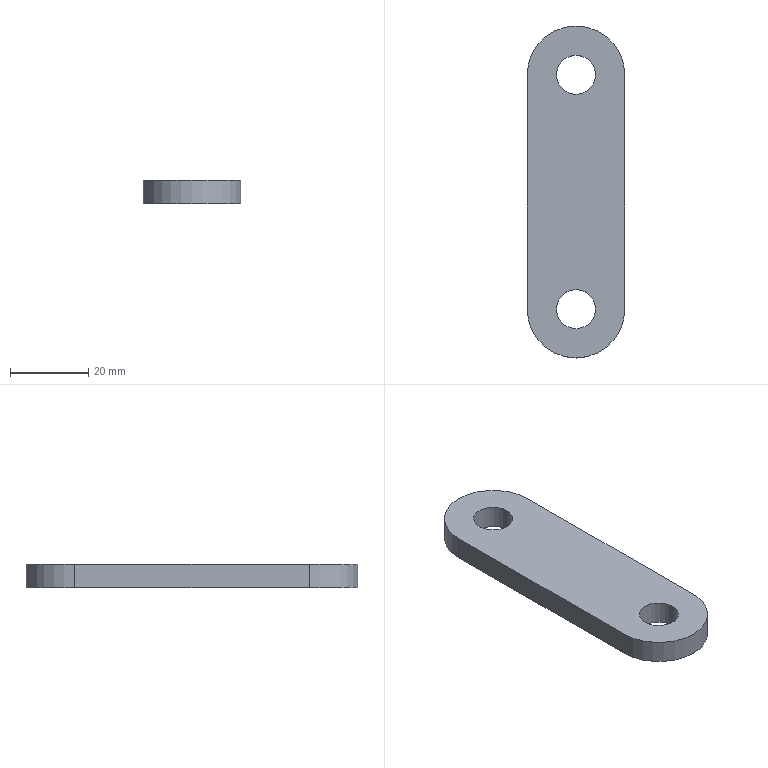Part | SolidWorks | features Extrusion 1 | 1 solid | 10 faces | box 25 x 85 x 6 mm | volume 11003 mm3 | cylinder 6 | plane 4 | commonest cylinder face diameters 10 x4 25 x2
STEP:
#1=CARTESIAN_POINT('',(-5.,60.,3.));
#2=VERTEX_POINT('',#1);
#3=CARTESIAN_POINT('',(5.,60.,3.));
#4=VERTEX_POINT('',#3);
#5=CARTESIAN_POINT('',(0.,60.,3.));
#6=DIRECTION('',(0.,0.,1.));
#7=DIRECTION('',(1.,0.,0.));
#8=AXIS2_PLACEMENT_3D('',#5,#6,#7);
#9=CIRCLE('',#8,5.);
#10=EDGE_CURVE('',#2,#4,#9,.T.);
#11=ORIENTED_EDGE('',*,*,#10,.T.);
#12=CARTESIAN_POINT('',(5.,60.,-3.));
#13=VERTEX_POINT('',#12);
#14=CARTESIAN_POINT('',(5.,60.,3.));
#15=DIRECTION('',(0.,0.,-1.));
#16=VECTOR('',#15,1000.);
#17=LINE('',#14,#16);
#18=EDGE_CURVE('',#4,#13,#17,.T.);
#19=ORIENTED_EDGE('',*,*,#18,.T.);
#20=CARTESIAN_POINT('',(-5.,60.,-3.));
#21=VERTEX_POINT('',#20);
#22=CARTESIAN_POINT('',(0.,60.,-3.));
#23=DIRECTION('',(0.,0.,1.));
#24=DIRECTION('',(1.,0.,0.));
#25=AXIS2_PLACEMENT_3D('',#22,#23,#24);
#26=CIRCLE('',#25,5.);
#27=EDGE_CURVE('',#21,#13,#26,.T.);
#28=ORIENTED_EDGE('',*,*,#27,.F.);
#29=CARTESIAN_POINT('',(-5.,60.,3.));
#30=DIRECTION('',(0.,0.,-1.));
#31=VECTOR('',#30,1000.);
#32=LINE('',#29,#31);
#33=EDGE_CURVE('',#2,#21,#32,.T.);
#34=ORIENTED_EDGE('',*,*,#33,.F.);
#35=EDGE_LOOP('',(#11,#19,#28,#34));
#36=FACE_OUTER_BOUND('',#35,.T.);
#37=CARTESIAN_POINT('',(0.,60.,3.));
#38=DIRECTION('',(0.,0.,-1.));
#39=DIRECTION('',(-1.,0.,0.));
#40=AXIS2_PLACEMENT_3D('',#37,#38,#39);
#41=CYLINDRICAL_SURFACE('',#40,5.);
#42=ADVANCED_FACE('',(#36),#41,.F.);
#43=CARTESIAN_POINT('',(-5.,0.,3.));
#44=VERTEX_POINT('',#43);
#45=CARTESIAN_POINT('',(5.,0.,3.));
#46=VERTEX_POINT('',#45);
#47=CARTESIAN_POINT('',(0.,0.,3.));
#48=DIRECTION('',(0.,0.,1.));
#49=DIRECTION('',(1.,0.,0.));
#50=AXIS2_PLACEMENT_3D('',#47,#48,#49);
#51=CIRCLE('',#50,5.);
#52=EDGE_CURVE('',#44,#46,#51,.T.);
#53=ORIENTED_EDGE('',*,*,#52,.T.);
#54=CARTESIAN_POINT('',(5.,0.,-3.));
#55=VERTEX_POINT('',#54);
#56=CARTESIAN_POINT('',(5.,0.,3.));
#57=DIRECTION('',(0.,0.,-1.));
#58=VECTOR('',#57,1000.);
#59=LINE('',#56,#58);
#60=EDGE_CURVE('',#46,#55,#59,.T.);
#61=ORIENTED_EDGE('',*,*,#60,.T.);
#62=CARTESIAN_POINT('',(-5.,0.,-3.));
#63=VERTEX_POINT('',#62);
#64=CARTESIAN_POINT('',(0.,0.,-3.));
#65=DIRECTION('',(0.,0.,1.));
#66=DIRECTION('',(1.,0.,0.));
#67=AXIS2_PLACEMENT_3D('',#64,#65,#66);
#68=CIRCLE('',#67,5.);
#69=EDGE_CURVE('',#63,#55,#68,.T.);
#70=ORIENTED_EDGE('',*,*,#69,.F.);
#71=CARTESIAN_POINT('',(-5.,0.,3.));
#72=DIRECTION('',(0.,0.,-1.));
#73=VECTOR('',#72,1000.);
#74=LINE('',#71,#73);
#75=EDGE_CURVE('',#44,#63,#74,.T.);
#76=ORIENTED_EDGE('',*,*,#75,.F.);
#77=EDGE_LOOP('',(#53,#61,#70,#76));
#78=FACE_OUTER_BOUND('',#77,.T.);
#79=CARTESIAN_POINT('',(0.,0.,3.));
#80=DIRECTION('',(0.,0.,-1.));
#81=DIRECTION('',(-1.,0.,0.));
#82=AXIS2_PLACEMENT_3D('',#79,#80,#81);
#83=CYLINDRICAL_SURFACE('',#82,5.);
#84=ADVANCED_FACE('',(#78),#83,.F.);
#85=ORIENTED_EDGE('',*,*,#52,.F.);
#86=CARTESIAN_POINT('',(0.,0.,3.));
#87=DIRECTION('',(0.,0.,1.));
#88=DIRECTION('',(1.,0.,0.));
#89=AXIS2_PLACEMENT_3D('',#86,#87,#88);
#90=CIRCLE('',#89,5.);
#91=EDGE_CURVE('',#46,#44,#90,.T.);
#92=ORIENTED_EDGE('',*,*,#91,.F.);
#93=EDGE_LOOP('',(#85,#92));
#94=FACE_BOUND('',#93,.T.);
#95=CARTESIAN_POINT('',(-12.5,0.,3.));
#96=VERTEX_POINT('',#95);
#97=CARTESIAN_POINT('',(12.5,0.,3.));
#98=VERTEX_POINT('',#97);
#99=CARTESIAN_POINT('',(0.,0.,3.));
#100=DIRECTION('',(0.,0.,1.));
#101=DIRECTION('',(1.,0.,0.));
#102=AXIS2_PLACEMENT_3D('',#99,#100,#101);
#103=CIRCLE('',#102,12.5);
#104=EDGE_CURVE('',#96,#98,#103,.T.);
#105=ORIENTED_EDGE('',*,*,#104,.T.);
#106=CARTESIAN_POINT('',(12.5,60.,3.));
#107=VERTEX_POINT('',#106);
#108=CARTESIAN_POINT('',(12.5,0.,3.));
#109=DIRECTION('',(0.,1.,0.));
#110=VECTOR('',#109,1000.);
#111=LINE('',#108,#110);
#112=EDGE_CURVE('',#98,#107,#111,.T.);
#113=ORIENTED_EDGE('',*,*,#112,.T.);
#114=CARTESIAN_POINT('',(-12.5,60.,3.));
#115=VERTEX_POINT('',#114);
#116=CARTESIAN_POINT('',(0.,60.,3.));
#117=DIRECTION('',(0.,0.,1.));
#118=DIRECTION('',(1.,0.,0.));
#119=AXIS2_PLACEMENT_3D('',#116,#117,#118);
#120=CIRCLE('',#119,12.5);
#121=EDGE_CURVE('',#107,#115,#120,.T.);
#122=ORIENTED_EDGE('',*,*,#121,.T.);
#123=CARTESIAN_POINT('',(-12.5,0.,3.));
#124=DIRECTION('',(0.,-1.,0.));
#125=VECTOR('',#124,1000.);
#126=LINE('',#123,#125);
#127=EDGE_CURVE('',#115,#96,#126,.T.);
#128=ORIENTED_EDGE('',*,*,#127,.T.);
#129=EDGE_LOOP('',(#105,#113,#122,#128));
#130=FACE_OUTER_BOUND('',#129,.T.);
#131=ORIENTED_EDGE('',*,*,#10,.F.);
#132=CARTESIAN_POINT('',(0.,60.,3.));
#133=DIRECTION('',(0.,0.,1.));
#134=DIRECTION('',(1.,0.,0.));
#135=AXIS2_PLACEMENT_3D('',#132,#133,#134);
#136=CIRCLE('',#135,5.);
#137=EDGE_CURVE('',#4,#2,#136,.T.);
#138=ORIENTED_EDGE('',*,*,#137,.F.);
#139=EDGE_LOOP('',(#131,#138));
#140=FACE_BOUND('',#139,.T.);
#141=CARTESIAN_POINT('',(0.,0.,3.));
#142=DIRECTION('',(0.,0.,1.));
#143=DIRECTION('',(1.,0.,0.));
#144=AXIS2_PLACEMENT_3D('',#141,#142,#143);
#145=PLANE('',#144);
#146=ADVANCED_FACE('',(#94,#130,#140),#145,.T.);
#147=CARTESIAN_POINT('',(-12.5,0.,-3.));
#148=VERTEX_POINT('',#147);
#149=CARTESIAN_POINT('',(12.5,0.,-3.));
#150=VERTEX_POINT('',#149);
#151=CARTESIAN_POINT('',(0.,0.,-3.));
#152=DIRECTION('',(0.,0.,1.));
#153=DIRECTION('',(1.,0.,0.));
#154=AXIS2_PLACEMENT_3D('',#151,#152,#153);
#155=CIRCLE('',#154,12.5);
#156=EDGE_CURVE('',#148,#150,#155,.T.);
#157=ORIENTED_EDGE('',*,*,#156,.F.);
#158=CARTESIAN_POINT('',(-12.5,60.,-3.));
#159=VERTEX_POINT('',#158);
#160=CARTESIAN_POINT('',(-12.5,0.,-3.));
#161=DIRECTION('',(0.,-1.,0.));
#162=VECTOR('',#161,1000.);
#163=LINE('',#160,#162);
#164=EDGE_CURVE('',#159,#148,#163,.T.);
#165=ORIENTED_EDGE('',*,*,#164,.F.);
#166=CARTESIAN_POINT('',(12.5,60.,-3.));
#167=VERTEX_POINT('',#166);
#168=CARTESIAN_POINT('',(0.,60.,-3.));
#169=DIRECTION('',(0.,0.,1.));
#170=DIRECTION('',(1.,0.,0.));
#171=AXIS2_PLACEMENT_3D('',#168,#169,#170);
#172=CIRCLE('',#171,12.5);
#173=EDGE_CURVE('',#167,#159,#172,.T.);
#174=ORIENTED_EDGE('',*,*,#173,.F.);
#175=CARTESIAN_POINT('',(12.5,0.,-3.));
#176=DIRECTION('',(0.,1.,0.));
#177=VECTOR('',#176,1000.);
#178=LINE('',#175,#177);
#179=EDGE_CURVE('',#150,#167,#178,.T.);
#180=ORIENTED_EDGE('',*,*,#179,.F.);
#181=EDGE_LOOP('',(#157,#165,#174,#180));
#182=FACE_OUTER_BOUND('',#181,.T.);
#183=ORIENTED_EDGE('',*,*,#69,.T.);
#184=CARTESIAN_POINT('',(0.,0.,-3.));
#185=DIRECTION('',(0.,0.,1.));
#186=DIRECTION('',(1.,0.,0.));
#187=AXIS2_PLACEMENT_3D('',#184,#185,#186);
#188=CIRCLE('',#187,5.);
#189=EDGE_CURVE('',#55,#63,#188,.T.);
#190=ORIENTED_EDGE('',*,*,#189,.T.);
#191=EDGE_LOOP('',(#183,#190));
#192=FACE_BOUND('',#191,.T.);
#193=ORIENTED_EDGE('',*,*,#27,.T.);
#194=CARTESIAN_POINT('',(0.,60.,-3.));
#195=DIRECTION('',(0.,0.,1.));
#196=DIRECTION('',(1.,0.,0.));
#197=AXIS2_PLACEMENT_3D('',#194,#195,#196);
#198=CIRCLE('',#197,5.);
#199=EDGE_CURVE('',#13,#21,#198,.T.);
#200=ORIENTED_EDGE('',*,*,#199,.T.);
#201=EDGE_LOOP('',(#193,#200));
#202=FACE_BOUND('',#201,.T.);
#203=CARTESIAN_POINT('',(0.,0.,-3.));
#204=DIRECTION('',(0.,0.,1.));
#205=DIRECTION('',(1.,0.,0.));
#206=AXIS2_PLACEMENT_3D('',#203,#204,#205);
#207=PLANE('',#206);
#208=ADVANCED_FACE('',(#182,#192,#202),#207,.F.);
#209=ORIENTED_EDGE('',*,*,#156,.T.);
#210=CARTESIAN_POINT('',(12.5,0.,3.));
#211=DIRECTION('',(0.,0.,-1.));
#212=VECTOR('',#211,1000.);
#213=LINE('',#210,#212);
#214=EDGE_CURVE('',#98,#150,#213,.T.);
#215=ORIENTED_EDGE('',*,*,#214,.F.);
#216=ORIENTED_EDGE('',*,*,#104,.F.);
#217=CARTESIAN_POINT('',(-12.5,0.,3.));
#218=DIRECTION('',(0.,0.,-1.));
#219=VECTOR('',#218,1000.);
#220=LINE('',#217,#219);
#221=EDGE_CURVE('',#96,#148,#220,.T.);
#222=ORIENTED_EDGE('',*,*,#221,.T.);
#223=EDGE_LOOP('',(#209,#215,#216,#222));
#224=FACE_OUTER_BOUND('',#223,.T.);
#225=CARTESIAN_POINT('',(0.,0.,3.));
#226=DIRECTION('',(0.,0.,-1.));
#227=DIRECTION('',(-1.,0.,0.));
#228=AXIS2_PLACEMENT_3D('',#225,#226,#227);
#229=CYLINDRICAL_SURFACE('',#228,12.5);
#230=ADVANCED_FACE('',(#224),#229,.T.);
#231=ORIENTED_EDGE('',*,*,#179,.T.);
#232=CARTESIAN_POINT('',(12.5,60.,3.));
#233=DIRECTION('',(0.,0.,-1.));
#234=VECTOR('',#233,1000.);
#235=LINE('',#232,#234);
#236=EDGE_CURVE('',#107,#167,#235,.T.);
#237=ORIENTED_EDGE('',*,*,#236,.F.);
#238=ORIENTED_EDGE('',*,*,#112,.F.);
#239=ORIENTED_EDGE('',*,*,#214,.T.);
#240=EDGE_LOOP('',(#231,#237,#238,#239));
#241=FACE_OUTER_BOUND('',#240,.T.);
#242=CARTESIAN_POINT('',(12.5,0.,3.));
#243=DIRECTION('',(-1.,0.,0.));
#244=DIRECTION('',(0.,0.,1.));
#245=AXIS2_PLACEMENT_3D('',#242,#243,#244);
#246=PLANE('',#245);
#247=ADVANCED_FACE('',(#241),#246,.F.);
#248=ORIENTED_EDGE('',*,*,#173,.T.);
#249=CARTESIAN_POINT('',(-12.5,60.,3.));
#250=DIRECTION('',(0.,0.,-1.));
#251=VECTOR('',#250,1000.);
#252=LINE('',#249,#251);
#253=EDGE_CURVE('',#115,#159,#252,.T.);
#254=ORIENTED_EDGE('',*,*,#253,.F.);
#255=ORIENTED_EDGE('',*,*,#121,.F.);
#256=ORIENTED_EDGE('',*,*,#236,.T.);
#257=EDGE_LOOP('',(#248,#254,#255,#256));
#258=FACE_OUTER_BOUND('',#257,.T.);
#259=CARTESIAN_POINT('',(0.,60.,3.));
#260=DIRECTION('',(0.,0.,-1.));
#261=DIRECTION('',(-1.,0.,0.));
#262=AXIS2_PLACEMENT_3D('',#259,#260,#261);
#263=CYLINDRICAL_SURFACE('',#262,12.5);
#264=ADVANCED_FACE('',(#258),#263,.T.);
#265=ORIENTED_EDGE('',*,*,#164,.T.);
#266=ORIENTED_EDGE('',*,*,#221,.F.);
#267=ORIENTED_EDGE('',*,*,#127,.F.);
#268=ORIENTED_EDGE('',*,*,#253,.T.);
#269=EDGE_LOOP('',(#265,#266,#267,#268));
#270=FACE_OUTER_BOUND('',#269,.T.);
#271=CARTESIAN_POINT('',(-12.5,0.,3.));
#272=DIRECTION('',(1.,0.,0.));
#273=DIRECTION('',(0.,0.,-1.));
#274=AXIS2_PLACEMENT_3D('',#271,#272,#273);
#275=PLANE('',#274);
#276=ADVANCED_FACE('',(#270),#275,.F.);
#277=ORIENTED_EDGE('',*,*,#60,.F.);
#278=ORIENTED_EDGE('',*,*,#91,.T.);
#279=ORIENTED_EDGE('',*,*,#75,.T.);
#280=ORIENTED_EDGE('',*,*,#189,.F.);
#281=EDGE_LOOP('',(#277,#278,#279,#280));
#282=FACE_OUTER_BOUND('',#281,.T.);
#283=CARTESIAN_POINT('',(0.,0.,3.));
#284=DIRECTION('',(0.,0.,-1.));
#285=DIRECTION('',(-1.,0.,0.));
#286=AXIS2_PLACEMENT_3D('',#283,#284,#285);
#287=CYLINDRICAL_SURFACE('',#286,5.);
#288=ADVANCED_FACE('',(#282),#287,.F.);
#289=ORIENTED_EDGE('',*,*,#18,.F.);
#290=ORIENTED_EDGE('',*,*,#137,.T.);
#291=ORIENTED_EDGE('',*,*,#33,.T.);
#292=ORIENTED_EDGE('',*,*,#199,.F.);
#293=EDGE_LOOP('',(#289,#290,#291,#292));
#294=FACE_OUTER_BOUND('',#293,.T.);
#295=CARTESIAN_POINT('',(0.,60.,3.));
#296=DIRECTION('',(0.,0.,-1.));
#297=DIRECTION('',(-1.,0.,0.));
#298=AXIS2_PLACEMENT_3D('',#295,#296,#297);
#299=CYLINDRICAL_SURFACE('',#298,5.);
#300=ADVANCED_FACE('',(#294),#299,.F.);
#301=CLOSED_SHELL('',(#42,#84,#146,#208,#230,#247,#264,#276,#288,#300));
#302=MANIFOLD_SOLID_BREP('',#301);
#303=CARTESIAN_POINT('',(0.,0.,0.));
#304=DIRECTION('',(0.,0.,1.));
#305=DIRECTION('',(1.,0.,0.));
#306=AXIS2_PLACEMENT_3D('',#303,#304,#305);
#307=(LENGTH_UNIT()NAMED_UNIT(*)SI_UNIT(.MILLI.,.METRE.));
#308=UNCERTAINTY_MEASURE_WITH_UNIT(LENGTH_MEASURE(0.00001),#307,'','');
#309=(NAMED_UNIT(*)PLANE_ANGLE_UNIT()SI_UNIT($,.RADIAN.));
#310=(NAMED_UNIT(*)SI_UNIT($,.STERADIAN.)SOLID_ANGLE_UNIT());
#311=(GEOMETRIC_REPRESENTATION_CONTEXT(3)GLOBAL_UNCERTAINTY_ASSIGNED_CONTEXT((#308))GLOBAL_UNIT_ASSIGNED_CONTEXT((#307,#309,#310))REPRESENTATION_CONTEXT('',''));
#312=ADVANCED_BREP_SHAPE_REPRESENTATION('',(#302,#306),#311);